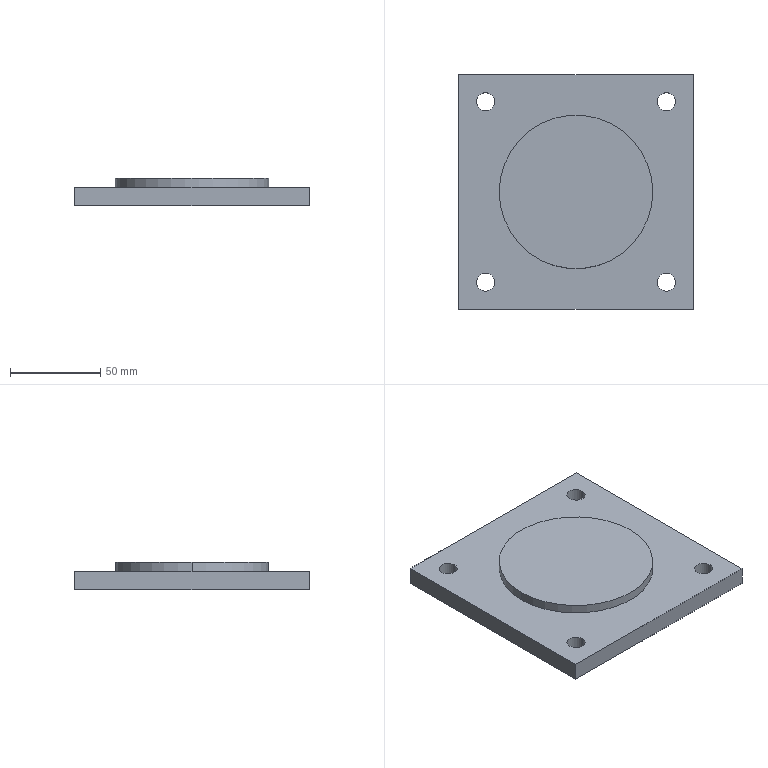Part | SolidWorks | features Cut 1, Extrusion 1, ICE 1 | 1 solid | 17 faces | box 130 x 130 x 15 mm | volume 194231 mm3 | cylinder 10 | plane 7 | commonest cylinder face diameters 10 x8 85 x2
STEP:
#1=CARTESIAN_POINT('',(45.,-50.,0.));
#2=VERTEX_POINT('',#1);
#3=CARTESIAN_POINT('',(55.,-50.,0.));
#4=VERTEX_POINT('',#3);
#5=CARTESIAN_POINT('',(50.,-50.,0.));
#6=DIRECTION('',(0.,0.,1.));
#7=DIRECTION('',(1.,0.,0.));
#8=AXIS2_PLACEMENT_3D('',#5,#6,#7);
#9=CIRCLE('',#8,5.);
#10=EDGE_CURVE('',#2,#4,#9,.T.);
#11=ORIENTED_EDGE('',*,*,#10,.F.);
#12=CARTESIAN_POINT('',(45.,-50.,10.));
#13=VERTEX_POINT('',#12);
#14=CARTESIAN_POINT('',(45.,-50.,-41.));
#15=DIRECTION('',(0.,0.,1.));
#16=VECTOR('',#15,1000.);
#17=LINE('',#14,#16);
#18=EDGE_CURVE('',#2,#13,#17,.T.);
#19=ORIENTED_EDGE('',*,*,#18,.T.);
#20=CARTESIAN_POINT('',(55.,-50.,10.));
#21=VERTEX_POINT('',#20);
#22=CARTESIAN_POINT('',(50.,-50.,10.));
#23=DIRECTION('',(0.,0.,1.));
#24=DIRECTION('',(1.,0.,0.));
#25=AXIS2_PLACEMENT_3D('',#22,#23,#24);
#26=CIRCLE('',#25,5.);
#27=EDGE_CURVE('',#13,#21,#26,.T.);
#28=ORIENTED_EDGE('',*,*,#27,.T.);
#29=CARTESIAN_POINT('',(55.,-50.,-41.));
#30=DIRECTION('',(0.,0.,1.));
#31=VECTOR('',#30,1000.);
#32=LINE('',#29,#31);
#33=EDGE_CURVE('',#4,#21,#32,.T.);
#34=ORIENTED_EDGE('',*,*,#33,.F.);
#35=EDGE_LOOP('',(#11,#19,#28,#34));
#36=FACE_OUTER_BOUND('',#35,.T.);
#37=CARTESIAN_POINT('',(50.,-50.,-41.));
#38=DIRECTION('',(0.,0.,1.));
#39=DIRECTION('',(1.,0.,0.));
#40=AXIS2_PLACEMENT_3D('',#37,#38,#39);
#41=CYLINDRICAL_SURFACE('',#40,5.);
#42=ADVANCED_FACE('',(#36),#41,.F.);
#43=CARTESIAN_POINT('',(-55.,-50.,0.));
#44=VERTEX_POINT('',#43);
#45=CARTESIAN_POINT('',(-45.,-50.,0.));
#46=VERTEX_POINT('',#45);
#47=CARTESIAN_POINT('',(-50.,-50.,0.));
#48=DIRECTION('',(0.,0.,1.));
#49=DIRECTION('',(1.,0.,0.));
#50=AXIS2_PLACEMENT_3D('',#47,#48,#49);
#51=CIRCLE('',#50,5.);
#52=EDGE_CURVE('',#44,#46,#51,.T.);
#53=ORIENTED_EDGE('',*,*,#52,.F.);
#54=CARTESIAN_POINT('',(-55.,-50.,10.));
#55=VERTEX_POINT('',#54);
#56=CARTESIAN_POINT('',(-55.,-50.,-41.));
#57=DIRECTION('',(0.,0.,1.));
#58=VECTOR('',#57,1000.);
#59=LINE('',#56,#58);
#60=EDGE_CURVE('',#44,#55,#59,.T.);
#61=ORIENTED_EDGE('',*,*,#60,.T.);
#62=CARTESIAN_POINT('',(-45.,-50.,10.));
#63=VERTEX_POINT('',#62);
#64=CARTESIAN_POINT('',(-50.,-50.,10.));
#65=DIRECTION('',(0.,0.,1.));
#66=DIRECTION('',(1.,0.,0.));
#67=AXIS2_PLACEMENT_3D('',#64,#65,#66);
#68=CIRCLE('',#67,5.);
#69=EDGE_CURVE('',#55,#63,#68,.T.);
#70=ORIENTED_EDGE('',*,*,#69,.T.);
#71=CARTESIAN_POINT('',(-45.,-50.,-41.));
#72=DIRECTION('',(0.,0.,1.));
#73=VECTOR('',#72,1000.);
#74=LINE('',#71,#73);
#75=EDGE_CURVE('',#46,#63,#74,.T.);
#76=ORIENTED_EDGE('',*,*,#75,.F.);
#77=EDGE_LOOP('',(#53,#61,#70,#76));
#78=FACE_OUTER_BOUND('',#77,.T.);
#79=CARTESIAN_POINT('',(-50.,-50.,-41.));
#80=DIRECTION('',(0.,0.,1.));
#81=DIRECTION('',(1.,0.,0.));
#82=AXIS2_PLACEMENT_3D('',#79,#80,#81);
#83=CYLINDRICAL_SURFACE('',#82,5.);
#84=ADVANCED_FACE('',(#78),#83,.F.);
#85=CARTESIAN_POINT('',(-55.,50.,0.));
#86=VERTEX_POINT('',#85);
#87=CARTESIAN_POINT('',(-45.,50.,0.));
#88=VERTEX_POINT('',#87);
#89=CARTESIAN_POINT('',(-50.,50.,0.));
#90=DIRECTION('',(0.,0.,1.));
#91=DIRECTION('',(1.,0.,0.));
#92=AXIS2_PLACEMENT_3D('',#89,#90,#91);
#93=CIRCLE('',#92,5.);
#94=EDGE_CURVE('',#86,#88,#93,.T.);
#95=ORIENTED_EDGE('',*,*,#94,.F.);
#96=CARTESIAN_POINT('',(-55.,50.,10.));
#97=VERTEX_POINT('',#96);
#98=CARTESIAN_POINT('',(-55.,50.,-41.));
#99=DIRECTION('',(0.,0.,1.));
#100=VECTOR('',#99,1000.);
#101=LINE('',#98,#100);
#102=EDGE_CURVE('',#86,#97,#101,.T.);
#103=ORIENTED_EDGE('',*,*,#102,.T.);
#104=CARTESIAN_POINT('',(-45.,50.,10.));
#105=VERTEX_POINT('',#104);
#106=CARTESIAN_POINT('',(-50.,50.,10.));
#107=DIRECTION('',(0.,0.,1.));
#108=DIRECTION('',(1.,0.,0.));
#109=AXIS2_PLACEMENT_3D('',#106,#107,#108);
#110=CIRCLE('',#109,5.);
#111=EDGE_CURVE('',#97,#105,#110,.T.);
#112=ORIENTED_EDGE('',*,*,#111,.T.);
#113=CARTESIAN_POINT('',(-45.,50.,-41.));
#114=DIRECTION('',(0.,0.,1.));
#115=VECTOR('',#114,1000.);
#116=LINE('',#113,#115);
#117=EDGE_CURVE('',#88,#105,#116,.T.);
#118=ORIENTED_EDGE('',*,*,#117,.F.);
#119=EDGE_LOOP('',(#95,#103,#112,#118));
#120=FACE_OUTER_BOUND('',#119,.T.);
#121=CARTESIAN_POINT('',(-50.,50.,-41.));
#122=DIRECTION('',(0.,0.,1.));
#123=DIRECTION('',(1.,0.,0.));
#124=AXIS2_PLACEMENT_3D('',#121,#122,#123);
#125=CYLINDRICAL_SURFACE('',#124,5.);
#126=ADVANCED_FACE('',(#120),#125,.F.);
#127=CARTESIAN_POINT('',(45.,50.,0.));
#128=VERTEX_POINT('',#127);
#129=CARTESIAN_POINT('',(55.,50.,0.));
#130=VERTEX_POINT('',#129);
#131=CARTESIAN_POINT('',(50.,50.,0.));
#132=DIRECTION('',(0.,0.,1.));
#133=DIRECTION('',(1.,0.,0.));
#134=AXIS2_PLACEMENT_3D('',#131,#132,#133);
#135=CIRCLE('',#134,5.);
#136=EDGE_CURVE('',#128,#130,#135,.T.);
#137=ORIENTED_EDGE('',*,*,#136,.F.);
#138=CARTESIAN_POINT('',(45.,50.,10.));
#139=VERTEX_POINT('',#138);
#140=CARTESIAN_POINT('',(45.,50.,-41.));
#141=DIRECTION('',(0.,0.,1.));
#142=VECTOR('',#141,1000.);
#143=LINE('',#140,#142);
#144=EDGE_CURVE('',#128,#139,#143,.T.);
#145=ORIENTED_EDGE('',*,*,#144,.T.);
#146=CARTESIAN_POINT('',(55.,50.,10.));
#147=VERTEX_POINT('',#146);
#148=CARTESIAN_POINT('',(50.,50.,10.));
#149=DIRECTION('',(0.,0.,1.));
#150=DIRECTION('',(1.,0.,0.));
#151=AXIS2_PLACEMENT_3D('',#148,#149,#150);
#152=CIRCLE('',#151,5.);
#153=EDGE_CURVE('',#139,#147,#152,.T.);
#154=ORIENTED_EDGE('',*,*,#153,.T.);
#155=CARTESIAN_POINT('',(55.,50.,-41.));
#156=DIRECTION('',(0.,0.,1.));
#157=VECTOR('',#156,1000.);
#158=LINE('',#155,#157);
#159=EDGE_CURVE('',#130,#147,#158,.T.);
#160=ORIENTED_EDGE('',*,*,#159,.F.);
#161=EDGE_LOOP('',(#137,#145,#154,#160));
#162=FACE_OUTER_BOUND('',#161,.T.);
#163=CARTESIAN_POINT('',(50.,50.,-41.));
#164=DIRECTION('',(0.,0.,1.));
#165=DIRECTION('',(1.,0.,0.));
#166=AXIS2_PLACEMENT_3D('',#163,#164,#165);
#167=CYLINDRICAL_SURFACE('',#166,5.);
#168=ADVANCED_FACE('',(#162),#167,.F.);
#169=CARTESIAN_POINT('',(42.5,0.,15.));
#170=VERTEX_POINT('',#169);
#171=CARTESIAN_POINT('',(-42.5,0.,15.));
#172=VERTEX_POINT('',#171);
#173=CARTESIAN_POINT('',(0.,0.,15.));
#174=DIRECTION('',(0.,0.,1.));
#175=DIRECTION('',(1.,0.,0.));
#176=AXIS2_PLACEMENT_3D('',#173,#174,#175);
#177=CIRCLE('',#176,42.5);
#178=EDGE_CURVE('',#170,#172,#177,.T.);
#179=ORIENTED_EDGE('',*,*,#178,.F.);
#180=CARTESIAN_POINT('',(42.5,0.,10.));
#181=VERTEX_POINT('',#180);
#182=CARTESIAN_POINT('',(42.5,0.,15.));
#183=DIRECTION('',(0.,0.,-1.));
#184=VECTOR('',#183,1000.);
#185=LINE('',#182,#184);
#186=EDGE_CURVE('',#170,#181,#185,.T.);
#187=ORIENTED_EDGE('',*,*,#186,.T.);
#188=CARTESIAN_POINT('',(-42.5,0.,10.));
#189=VERTEX_POINT('',#188);
#190=CARTESIAN_POINT('',(0.,0.,10.));
#191=DIRECTION('',(0.,0.,1.));
#192=DIRECTION('',(1.,0.,0.));
#193=AXIS2_PLACEMENT_3D('',#190,#191,#192);
#194=CIRCLE('',#193,42.5);
#195=EDGE_CURVE('',#181,#189,#194,.T.);
#196=ORIENTED_EDGE('',*,*,#195,.T.);
#197=CARTESIAN_POINT('',(-42.5,0.,15.));
#198=DIRECTION('',(0.,0.,-1.));
#199=VECTOR('',#198,1000.);
#200=LINE('',#197,#199);
#201=EDGE_CURVE('',#172,#189,#200,.T.);
#202=ORIENTED_EDGE('',*,*,#201,.F.);
#203=EDGE_LOOP('',(#179,#187,#196,#202));
#204=FACE_OUTER_BOUND('',#203,.T.);
#205=CARTESIAN_POINT('',(0.,0.,15.));
#206=DIRECTION('',(0.,0.,-1.));
#207=DIRECTION('',(-1.,0.,0.));
#208=AXIS2_PLACEMENT_3D('',#205,#206,#207);
#209=CYLINDRICAL_SURFACE('',#208,42.5);
#210=ADVANCED_FACE('',(#204),#209,.T.);
#211=CARTESIAN_POINT('',(65.,-65.,0.));
#212=VERTEX_POINT('',#211);
#213=CARTESIAN_POINT('',(65.,65.,0.));
#214=VERTEX_POINT('',#213);
#215=CARTESIAN_POINT('',(65.,65.,0.));
#216=DIRECTION('',(0.,1.,0.));
#217=VECTOR('',#216,1000.);
#218=LINE('',#215,#217);
#219=EDGE_CURVE('',#212,#214,#218,.T.);
#220=ORIENTED_EDGE('',*,*,#219,.T.);
#221=CARTESIAN_POINT('',(65.,65.,10.));
#222=VERTEX_POINT('',#221);
#223=CARTESIAN_POINT('',(65.,65.,10.));
#224=DIRECTION('',(0.,0.,-1.));
#225=VECTOR('',#224,1000.);
#226=LINE('',#223,#225);
#227=EDGE_CURVE('',#222,#214,#226,.T.);
#228=ORIENTED_EDGE('',*,*,#227,.F.);
#229=CARTESIAN_POINT('',(65.,-65.,10.));
#230=VERTEX_POINT('',#229);
#231=CARTESIAN_POINT('',(65.,65.,10.));
#232=DIRECTION('',(0.,1.,0.));
#233=VECTOR('',#232,1000.);
#234=LINE('',#231,#233);
#235=EDGE_CURVE('',#230,#222,#234,.T.);
#236=ORIENTED_EDGE('',*,*,#235,.F.);
#237=CARTESIAN_POINT('',(65.,-65.,10.));
#238=DIRECTION('',(0.,0.,-1.));
#239=VECTOR('',#238,1000.);
#240=LINE('',#237,#239);
#241=EDGE_CURVE('',#230,#212,#240,.T.);
#242=ORIENTED_EDGE('',*,*,#241,.T.);
#243=EDGE_LOOP('',(#220,#228,#236,#242));
#244=FACE_OUTER_BOUND('',#243,.T.);
#245=CARTESIAN_POINT('',(65.,65.,10.));
#246=DIRECTION('',(-1.,0.,0.));
#247=DIRECTION('',(0.,0.,1.));
#248=AXIS2_PLACEMENT_3D('',#245,#246,#247);
#249=PLANE('',#248);
#250=ADVANCED_FACE('',(#244),#249,.F.);
#251=CARTESIAN_POINT('',(-65.,65.,0.));
#252=VERTEX_POINT('',#251);
#253=CARTESIAN_POINT('',(-65.,65.,0.));
#254=DIRECTION('',(-1.,0.,0.));
#255=VECTOR('',#254,1000.);
#256=LINE('',#253,#255);
#257=EDGE_CURVE('',#214,#252,#256,.T.);
#258=ORIENTED_EDGE('',*,*,#257,.T.);
#259=CARTESIAN_POINT('',(-65.,65.,10.));
#260=VERTEX_POINT('',#259);
#261=CARTESIAN_POINT('',(-65.,65.,10.));
#262=DIRECTION('',(0.,0.,-1.));
#263=VECTOR('',#262,1000.);
#264=LINE('',#261,#263);
#265=EDGE_CURVE('',#260,#252,#264,.T.);
#266=ORIENTED_EDGE('',*,*,#265,.F.);
#267=CARTESIAN_POINT('',(-65.,65.,10.));
#268=DIRECTION('',(-1.,0.,0.));
#269=VECTOR('',#268,1000.);
#270=LINE('',#267,#269);
#271=EDGE_CURVE('',#222,#260,#270,.T.);
#272=ORIENTED_EDGE('',*,*,#271,.F.);
#273=ORIENTED_EDGE('',*,*,#227,.T.);
#274=EDGE_LOOP('',(#258,#266,#272,#273));
#275=FACE_OUTER_BOUND('',#274,.T.);
#276=CARTESIAN_POINT('',(-65.,65.,10.));
#277=DIRECTION('',(0.,-1.,0.));
#278=DIRECTION('',(0.,0.,-1.));
#279=AXIS2_PLACEMENT_3D('',#276,#277,#278);
#280=PLANE('',#279);
#281=ADVANCED_FACE('',(#275),#280,.F.);
#282=CARTESIAN_POINT('',(-65.,-65.,0.));
#283=VERTEX_POINT('',#282);
#284=CARTESIAN_POINT('',(-65.,65.,0.));
#285=DIRECTION('',(0.,-1.,0.));
#286=VECTOR('',#285,1000.);
#287=LINE('',#284,#286);
#288=EDGE_CURVE('',#252,#283,#287,.T.);
#289=ORIENTED_EDGE('',*,*,#288,.T.);
#290=CARTESIAN_POINT('',(-65.,-65.,10.));
#291=VERTEX_POINT('',#290);
#292=CARTESIAN_POINT('',(-65.,-65.,10.));
#293=DIRECTION('',(0.,0.,-1.));
#294=VECTOR('',#293,1000.);
#295=LINE('',#292,#294);
#296=EDGE_CURVE('',#291,#283,#295,.T.);
#297=ORIENTED_EDGE('',*,*,#296,.F.);
#298=CARTESIAN_POINT('',(-65.,65.,10.));
#299=DIRECTION('',(0.,-1.,0.));
#300=VECTOR('',#299,1000.);
#301=LINE('',#298,#300);
#302=EDGE_CURVE('',#260,#291,#301,.T.);
#303=ORIENTED_EDGE('',*,*,#302,.F.);
#304=ORIENTED_EDGE('',*,*,#265,.T.);
#305=EDGE_LOOP('',(#289,#297,#303,#304));
#306=FACE_OUTER_BOUND('',#305,.T.);
#307=CARTESIAN_POINT('',(-65.,65.,10.));
#308=DIRECTION('',(1.,0.,0.));
#309=DIRECTION('',(0.,1.,0.));
#310=AXIS2_PLACEMENT_3D('',#307,#308,#309);
#311=PLANE('',#310);
#312=ADVANCED_FACE('',(#306),#311,.F.);
#313=CARTESIAN_POINT('',(-65.,-65.,0.));
#314=DIRECTION('',(1.,0.,0.));
#315=VECTOR('',#314,1000.);
#316=LINE('',#313,#315);
#317=EDGE_CURVE('',#283,#212,#316,.T.);
#318=ORIENTED_EDGE('',*,*,#317,.T.);
#319=ORIENTED_EDGE('',*,*,#241,.F.);
#320=CARTESIAN_POINT('',(-65.,-65.,10.));
#321=DIRECTION('',(1.,0.,0.));
#322=VECTOR('',#321,1000.);
#323=LINE('',#320,#322);
#324=EDGE_CURVE('',#291,#230,#323,.T.);
#325=ORIENTED_EDGE('',*,*,#324,.F.);
#326=ORIENTED_EDGE('',*,*,#296,.T.);
#327=EDGE_LOOP('',(#318,#319,#325,#326));
#328=FACE_OUTER_BOUND('',#327,.T.);
#329=CARTESIAN_POINT('',(-65.,-65.,10.));
#330=DIRECTION('',(0.,1.,0.));
#331=DIRECTION('',(0.,0.,1.));
#332=AXIS2_PLACEMENT_3D('',#329,#330,#331);
#333=PLANE('',#332);
#334=ADVANCED_FACE('',(#328),#333,.F.);
#335=CARTESIAN_POINT('',(50.,-50.,10.));
#336=DIRECTION('',(0.,0.,1.));
#337=DIRECTION('',(1.,0.,0.));
#338=AXIS2_PLACEMENT_3D('',#335,#336,#337);
#339=CIRCLE('',#338,5.);
#340=EDGE_CURVE('',#21,#13,#339,.T.);
#341=ORIENTED_EDGE('',*,*,#340,.F.);
#342=ORIENTED_EDGE('',*,*,#27,.F.);
#343=EDGE_LOOP('',(#341,#342));
#344=FACE_BOUND('',#343,.T.);
#345=CARTESIAN_POINT('',(-50.,-50.,10.));
#346=DIRECTION('',(0.,0.,1.));
#347=DIRECTION('',(1.,0.,0.));
#348=AXIS2_PLACEMENT_3D('',#345,#346,#347);
#349=CIRCLE('',#348,5.);
#350=EDGE_CURVE('',#63,#55,#349,.T.);
#351=ORIENTED_EDGE('',*,*,#350,.F.);
#352=ORIENTED_EDGE('',*,*,#69,.F.);
#353=EDGE_LOOP('',(#351,#352));
#354=FACE_BOUND('',#353,.T.);
#355=CARTESIAN_POINT('',(-50.,50.,10.));
#356=DIRECTION('',(0.,0.,1.));
#357=DIRECTION('',(1.,0.,0.));
#358=AXIS2_PLACEMENT_3D('',#355,#356,#357);
#359=CIRCLE('',#358,5.);
#360=EDGE_CURVE('',#105,#97,#359,.T.);
#361=ORIENTED_EDGE('',*,*,#360,.F.);
#362=ORIENTED_EDGE('',*,*,#111,.F.);
#363=EDGE_LOOP('',(#361,#362));
#364=FACE_BOUND('',#363,.T.);
#365=CARTESIAN_POINT('',(50.,50.,10.));
#366=DIRECTION('',(0.,0.,1.));
#367=DIRECTION('',(1.,0.,0.));
#368=AXIS2_PLACEMENT_3D('',#365,#366,#367);
#369=CIRCLE('',#368,5.);
#370=EDGE_CURVE('',#147,#139,#369,.T.);
#371=ORIENTED_EDGE('',*,*,#370,.F.);
#372=ORIENTED_EDGE('',*,*,#153,.F.);
#373=EDGE_LOOP('',(#371,#372));
#374=FACE_BOUND('',#373,.T.);
#375=CARTESIAN_POINT('',(0.,0.,10.));
#376=DIRECTION('',(0.,0.,1.));
#377=DIRECTION('',(1.,0.,0.));
#378=AXIS2_PLACEMENT_3D('',#375,#376,#377);
#379=CIRCLE('',#378,42.5);
#380=EDGE_CURVE('',#189,#181,#379,.T.);
#381=ORIENTED_EDGE('',*,*,#380,.F.);
#382=ORIENTED_EDGE('',*,*,#195,.F.);
#383=EDGE_LOOP('',(#381,#382));
#384=FACE_BOUND('',#383,.T.);
#385=ORIENTED_EDGE('',*,*,#235,.T.);
#386=ORIENTED_EDGE('',*,*,#271,.T.);
#387=ORIENTED_EDGE('',*,*,#302,.T.);
#388=ORIENTED_EDGE('',*,*,#324,.T.);
#389=EDGE_LOOP('',(#385,#386,#387,#388));
#390=FACE_OUTER_BOUND('',#389,.T.);
#391=CARTESIAN_POINT('',(0.,0.,10.));
#392=DIRECTION('',(0.,0.,1.));
#393=DIRECTION('',(1.,0.,0.));
#394=AXIS2_PLACEMENT_3D('',#391,#392,#393);
#395=PLANE('',#394);
#396=ADVANCED_FACE('',(#344,#354,#364,#374,#384,#390),#395,.T.);
#397=CARTESIAN_POINT('',(50.,-50.,0.));
#398=DIRECTION('',(0.,0.,1.));
#399=DIRECTION('',(1.,0.,0.));
#400=AXIS2_PLACEMENT_3D('',#397,#398,#399);
#401=CIRCLE('',#400,5.);
#402=EDGE_CURVE('',#4,#2,#401,.T.);
#403=ORIENTED_EDGE('',*,*,#402,.T.);
#404=ORIENTED_EDGE('',*,*,#10,.T.);
#405=EDGE_LOOP('',(#403,#404));
#406=FACE_BOUND('',#405,.T.);
#407=CARTESIAN_POINT('',(-50.,-50.,0.));
#408=DIRECTION('',(0.,0.,1.));
#409=DIRECTION('',(1.,0.,0.));
#410=AXIS2_PLACEMENT_3D('',#407,#408,#409);
#411=CIRCLE('',#410,5.);
#412=EDGE_CURVE('',#46,#44,#411,.T.);
#413=ORIENTED_EDGE('',*,*,#412,.T.);
#414=ORIENTED_EDGE('',*,*,#52,.T.);
#415=EDGE_LOOP('',(#413,#414));
#416=FACE_BOUND('',#415,.T.);
#417=CARTESIAN_POINT('',(-50.,50.,0.));
#418=DIRECTION('',(0.,0.,1.));
#419=DIRECTION('',(1.,0.,0.));
#420=AXIS2_PLACEMENT_3D('',#417,#418,#419);
#421=CIRCLE('',#420,5.);
#422=EDGE_CURVE('',#88,#86,#421,.T.);
#423=ORIENTED_EDGE('',*,*,#422,.T.);
#424=ORIENTED_EDGE('',*,*,#94,.T.);
#425=EDGE_LOOP('',(#423,#424));
#426=FACE_BOUND('',#425,.T.);
#427=CARTESIAN_POINT('',(50.,50.,0.));
#428=DIRECTION('',(0.,0.,1.));
#429=DIRECTION('',(1.,0.,0.));
#430=AXIS2_PLACEMENT_3D('',#427,#428,#429);
#431=CIRCLE('',#430,5.);
#432=EDGE_CURVE('',#130,#128,#431,.T.);
#433=ORIENTED_EDGE('',*,*,#432,.T.);
#434=ORIENTED_EDGE('',*,*,#136,.T.);
#435=EDGE_LOOP('',(#433,#434));
#436=FACE_BOUND('',#435,.T.);
#437=ORIENTED_EDGE('',*,*,#219,.F.);
#438=ORIENTED_EDGE('',*,*,#317,.F.);
#439=ORIENTED_EDGE('',*,*,#288,.F.);
#440=ORIENTED_EDGE('',*,*,#257,.F.);
#441=EDGE_LOOP('',(#437,#438,#439,#440));
#442=FACE_OUTER_BOUND('',#441,.T.);
#443=CARTESIAN_POINT('',(0.,0.,0.));
#444=DIRECTION('',(0.,0.,1.));
#445=DIRECTION('',(1.,0.,0.));
#446=AXIS2_PLACEMENT_3D('',#443,#444,#445);
#447=PLANE('',#446);
#448=ADVANCED_FACE('',(#406,#416,#426,#436,#442),#447,.F.);
#449=ORIENTED_EDGE('',*,*,#186,.F.);
#450=CARTESIAN_POINT('',(0.,0.,15.));
#451=DIRECTION('',(0.,0.,1.));
#452=DIRECTION('',(1.,0.,0.));
#453=AXIS2_PLACEMENT_3D('',#450,#451,#452);
#454=CIRCLE('',#453,42.5);
#455=EDGE_CURVE('',#172,#170,#454,.T.);
#456=ORIENTED_EDGE('',*,*,#455,.F.);
#457=ORIENTED_EDGE('',*,*,#201,.T.);
#458=ORIENTED_EDGE('',*,*,#380,.T.);
#459=EDGE_LOOP('',(#449,#456,#457,#458));
#460=FACE_OUTER_BOUND('',#459,.T.);
#461=CARTESIAN_POINT('',(0.,0.,15.));
#462=DIRECTION('',(0.,0.,-1.));
#463=DIRECTION('',(-1.,0.,0.));
#464=AXIS2_PLACEMENT_3D('',#461,#462,#463);
#465=CYLINDRICAL_SURFACE('',#464,42.5);
#466=ADVANCED_FACE('',(#460),#465,.T.);
#467=ORIENTED_EDGE('',*,*,#455,.T.);
#468=ORIENTED_EDGE('',*,*,#178,.T.);
#469=EDGE_LOOP('',(#467,#468));
#470=FACE_OUTER_BOUND('',#469,.T.);
#471=CARTESIAN_POINT('',(0.,0.,15.));
#472=DIRECTION('',(0.,0.,1.));
#473=DIRECTION('',(1.,0.,0.));
#474=AXIS2_PLACEMENT_3D('',#471,#472,#473);
#475=PLANE('',#474);
#476=ADVANCED_FACE('',(#470),#475,.T.);
#477=ORIENTED_EDGE('',*,*,#144,.F.);
#478=ORIENTED_EDGE('',*,*,#432,.F.);
#479=ORIENTED_EDGE('',*,*,#159,.T.);
#480=ORIENTED_EDGE('',*,*,#370,.T.);
#481=EDGE_LOOP('',(#477,#478,#479,#480));
#482=FACE_OUTER_BOUND('',#481,.T.);
#483=CARTESIAN_POINT('',(50.,50.,-41.));
#484=DIRECTION('',(0.,0.,1.));
#485=DIRECTION('',(1.,0.,0.));
#486=AXIS2_PLACEMENT_3D('',#483,#484,#485);
#487=CYLINDRICAL_SURFACE('',#486,5.);
#488=ADVANCED_FACE('',(#482),#487,.F.);
#489=ORIENTED_EDGE('',*,*,#102,.F.);
#490=ORIENTED_EDGE('',*,*,#422,.F.);
#491=ORIENTED_EDGE('',*,*,#117,.T.);
#492=ORIENTED_EDGE('',*,*,#360,.T.);
#493=EDGE_LOOP('',(#489,#490,#491,#492));
#494=FACE_OUTER_BOUND('',#493,.T.);
#495=CARTESIAN_POINT('',(-50.,50.,-41.));
#496=DIRECTION('',(0.,0.,1.));
#497=DIRECTION('',(1.,0.,0.));
#498=AXIS2_PLACEMENT_3D('',#495,#496,#497);
#499=CYLINDRICAL_SURFACE('',#498,5.);
#500=ADVANCED_FACE('',(#494),#499,.F.);
#501=ORIENTED_EDGE('',*,*,#60,.F.);
#502=ORIENTED_EDGE('',*,*,#412,.F.);
#503=ORIENTED_EDGE('',*,*,#75,.T.);
#504=ORIENTED_EDGE('',*,*,#350,.T.);
#505=EDGE_LOOP('',(#501,#502,#503,#504));
#506=FACE_OUTER_BOUND('',#505,.T.);
#507=CARTESIAN_POINT('',(-50.,-50.,-41.));
#508=DIRECTION('',(0.,0.,1.));
#509=DIRECTION('',(1.,0.,0.));
#510=AXIS2_PLACEMENT_3D('',#507,#508,#509);
#511=CYLINDRICAL_SURFACE('',#510,5.);
#512=ADVANCED_FACE('',(#506),#511,.F.);
#513=ORIENTED_EDGE('',*,*,#18,.F.);
#514=ORIENTED_EDGE('',*,*,#402,.F.);
#515=ORIENTED_EDGE('',*,*,#33,.T.);
#516=ORIENTED_EDGE('',*,*,#340,.T.);
#517=EDGE_LOOP('',(#513,#514,#515,#516));
#518=FACE_OUTER_BOUND('',#517,.T.);
#519=CARTESIAN_POINT('',(50.,-50.,-41.));
#520=DIRECTION('',(0.,0.,1.));
#521=DIRECTION('',(1.,0.,0.));
#522=AXIS2_PLACEMENT_3D('',#519,#520,#521);
#523=CYLINDRICAL_SURFACE('',#522,5.);
#524=ADVANCED_FACE('',(#518),#523,.F.);
#525=CLOSED_SHELL('',(#42,#84,#126,#168,#210,#250,#281,#312,#334,#396,#448,#466,#476,#488,#500,#512,#524));
#526=MANIFOLD_SOLID_BREP('',#525);
#527=CARTESIAN_POINT('',(0.,0.,0.));
#528=DIRECTION('',(0.,0.,1.));
#529=DIRECTION('',(1.,0.,0.));
#530=AXIS2_PLACEMENT_3D('',#527,#528,#529);
#531=(LENGTH_UNIT()NAMED_UNIT(*)SI_UNIT(.MILLI.,.METRE.));
#532=UNCERTAINTY_MEASURE_WITH_UNIT(LENGTH_MEASURE(0.00001),#531,'','');
#533=(NAMED_UNIT(*)PLANE_ANGLE_UNIT()SI_UNIT($,.RADIAN.));
#534=(NAMED_UNIT(*)SI_UNIT($,.STERADIAN.)SOLID_ANGLE_UNIT());
#535=(GEOMETRIC_REPRESENTATION_CONTEXT(3)GLOBAL_UNCERTAINTY_ASSIGNED_CONTEXT((#532))GLOBAL_UNIT_ASSIGNED_CONTEXT((#531,#533,#534))REPRESENTATION_CONTEXT('',''));
#536=ADVANCED_BREP_SHAPE_REPRESENTATION('',(#526,#530),#535);